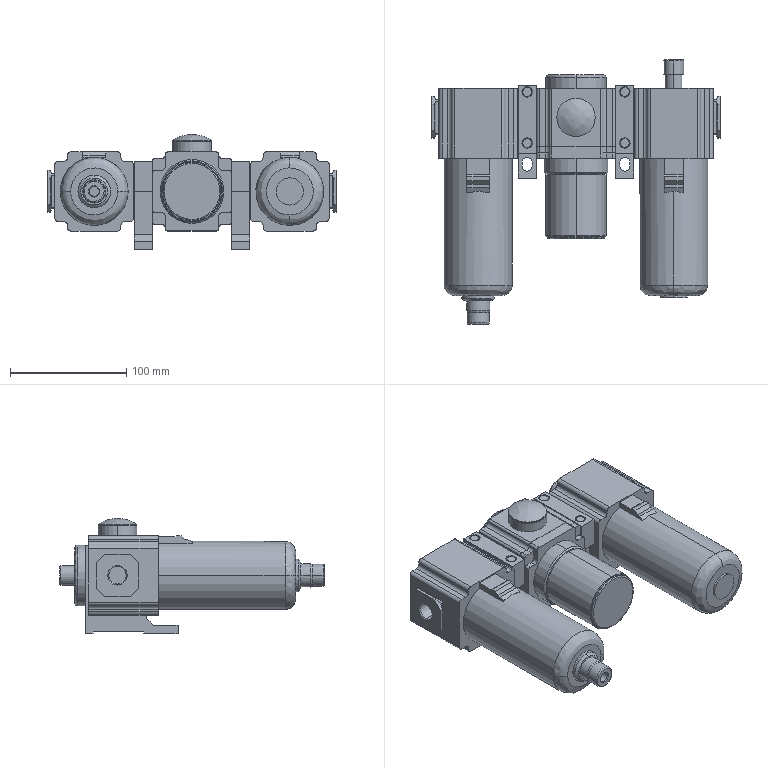Part | STEP file | pneumatic FRL unit GAC40010AS | 5 solids | 465 faces | box 248 x 227 x 99 mm | volume 1724530 mm3 | plane 278 | cylinder 134 | spline 31 | cone 22 | commonest cylinder face diameters 6 x36 4 x20 14.95 x12 8.5 x8 9 x8 36.2 x8